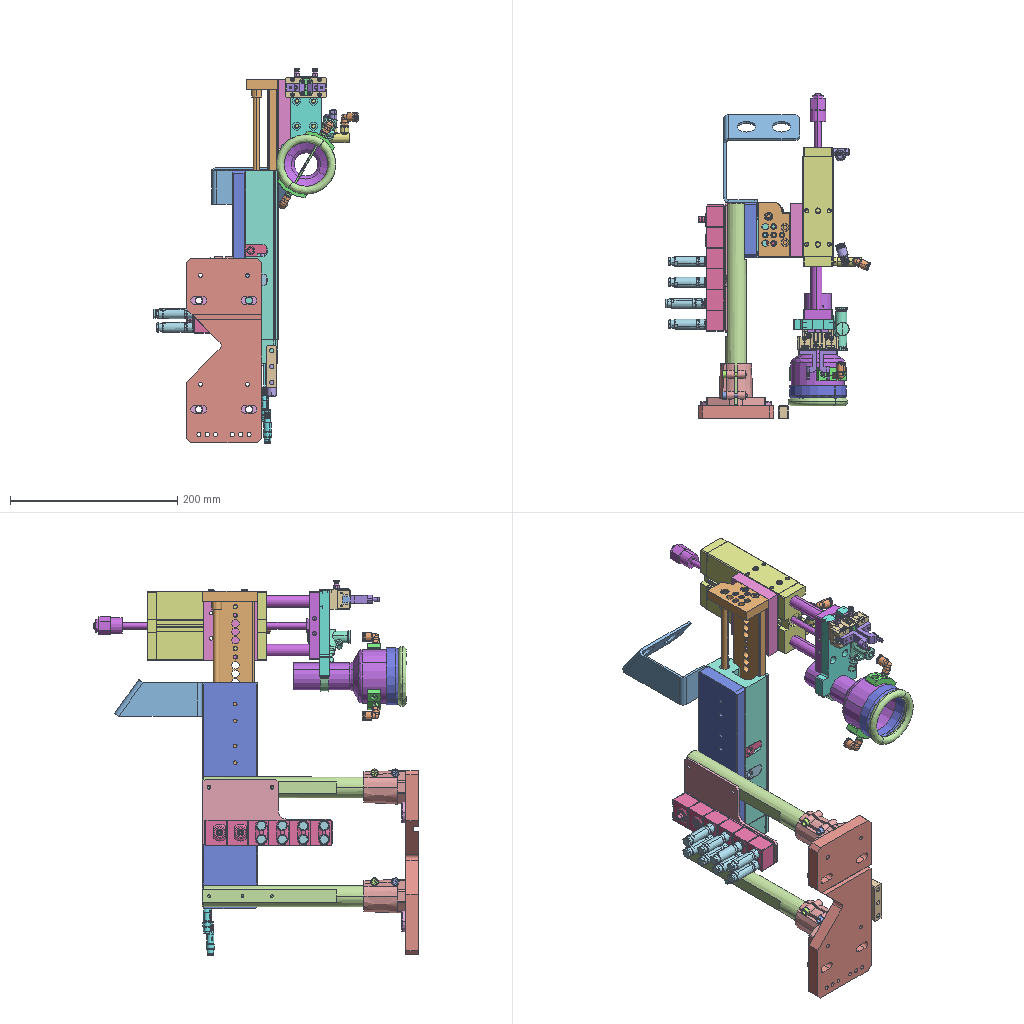Assembly | SolidWorks | 44 different items | 71 placed | box 245 x 388 x 448 mm
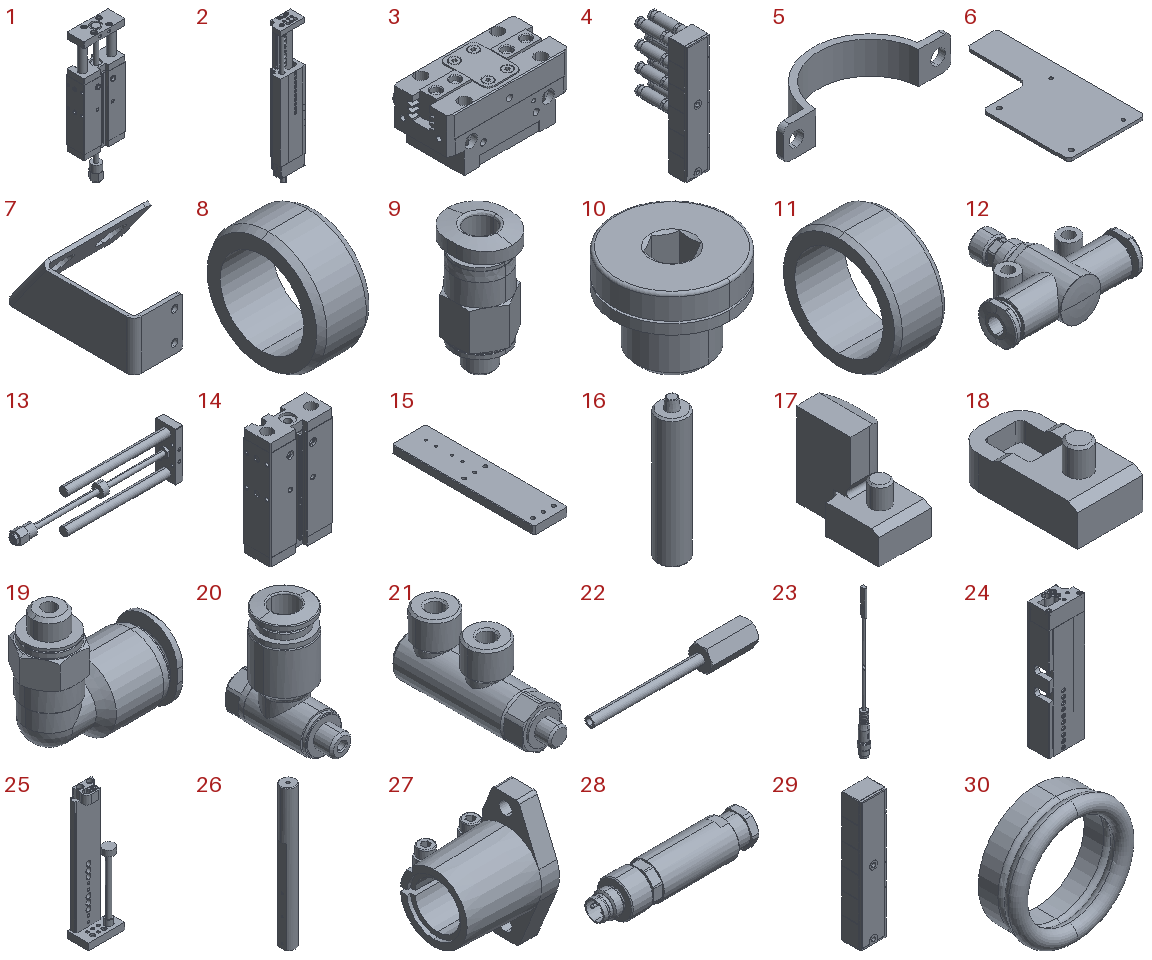Parts list (item | name | quantity | parent item | size | volume | features):
1 | (subassembly) | x1 | - | 84.4 x 37.9 x 271.9 mm | 422622 mm3 | -
2 | (subassembly) | x1 | - | 66 x 40 x 379 mm | 460415 mm3 | -
3 | (subassembly) | x1 | - | 50 x 34.8 x 24.7 mm | 23663 mm3 | -
4 | (subassembly) | x1 | - | 30 x 71.1 x 151 mm | 135395 mm3 | -
5 | - | x1 | - | 52 x 17 x 10 mm | 1282 mm3 | features ExtruThin 1, Fillet 1, HoleWzd 1
6 | - | x1 | - | 80 x 155 x 3 mm | 27690 mm3 | features HoleWzd 2, Chamfer 1, Extrusion 1, Fillet 1, ICE 1
7 | - | x1 | - | 91 x 104.854 x 43.527 mm | 25604 mm3 | features Fillet 2, ICE 2, EdgeFlange 1, FlatPattern 1, HoleWzd 1, SMBaseFlange 1, SheetMetal 1
8 | - | x4 | in 1 | 4 x 9 x 9 mm | 121.796 mm3 | features RefAxis 9, 3DProfileFeature 3, Revolution 1
9 | - | x2 | in 3 | 6 x 7 x 13.3 mm | 216.387 mm3 | features BaseBody 1
10 | - | x2 | in 2 | 8 x 8 x 6.3 mm | 181.471 mm3 | features RefAxis 6, 3DProfileFeature 2, ICE 1, Revolution 1
11 | - | x2 | in 1 | 3 x 7 x 7 mm | 48.144 mm3 | features RefAxis 9, 3DProfileFeature 3, Revolution 1
12 | - | x1 | - | 51.6 x 40.42 x 16.166 mm | 11359 mm3 | features BaseBody 1
13 | - | x1 | in 1 | 270 x 34 x 81 mm | 107228 mm3 | features RefAxis 9, RevCut 7, Revolution 6, ICE 4, 3DProfileFeature 3, HoleWzd 2, Extrusion 1
14 | - | x1 | in 1 | 83 x 36 x 142 mm | 314811 mm3 | features RefAxis 33, RevCut 25, 3DProfileFeature 11, ICE 4, Extrusion 1
15 | - | x1 | - | 66 x 270 x 15 mm | 261133 mm3 | features Chamfer 2, HoleWzd 2, ICE 2, Extrusion 1, MoveFace 1
16 | - | x2 | in 2 | 12 x 12 x 58.2 mm | 5676 mm3 | features RefAxis 21, 3DProfileFeature 7, Revolution 3, ICE 2, RevCut 2
17 | - | x1 | in 2 | 14 x 26.1 x 22.4 mm | 4263 mm3 | features ICE 6, RefAxis 3, 3DProfileFeature 1, Extrusion 1, RevCut 1, Revolution 1
18 | - | x1 | in 2 | 13.9 x 26.1 x 13.7 mm | 2228 mm3 | features ICE 4, RefAxis 3, 3DProfileFeature 1, Extrusion 1, RevCut 1, Revolution 1
19 | - | x3 | - | 20.919 x 10.5 x 20.4 mm | 1362 mm3 | features RefAxis 9, 3DProfileFeature 3, Revolution 3, ICE 2, RevCut 2
20 | - | x2 | - | 11.8 x 24.4 x 26.45 mm | 2431 mm3 | features BaseBody 1
21 | - | x1 | - | 11 x 39 x 19 mm | 4357 mm3 | features BaseBody 1
22 | - | x2 | - | 50 x 8.083 x 7 mm | 663.119 mm3 | features BaseBody 1
23 | - | x2 | - | 9.6 x 9.6 x 150.7 mm | 2540 mm3 | features Attribute 301, BaseBody 5, ICE 1
24 | - | x1 | in 2 | 66 x 39.6 x 230 mm | 297307 mm3 | features RefAxis 57, RevCut 21, 3DProfileFeature 19, ICE 16, Revolution 4, Extrusion 1
25 | - | x1 | in 2 | 65 x 38.5 x 229 mm | 144902 mm3 | features RevCut 22, RefAxis 18, ICE 12, 3DProfileFeature 6, Revolution 2, Extrusion 1
26 | - | x2 | - | 25 x 25 x 243 mm | 111932 mm3 | features HoleWzd 3, ICE 3, Chamfer 1, Extrusion 1
27 | - | x2 | - | 50 x 42 x 70 mm | 41488 mm3 | features BaseBody 3
28 | - | x8 | in 4 | 50.1 x 12 x 12 mm | 4699 mm3 | features BaseBody 1
29 | - | x1 | in 4 | 30 x 31.5 x 151 mm | 97801 mm3 | features BaseBody 1
30 | - | x1 | - | 71.5 x 24 x 71.5 mm | 15845 mm3 | features Sweep 2
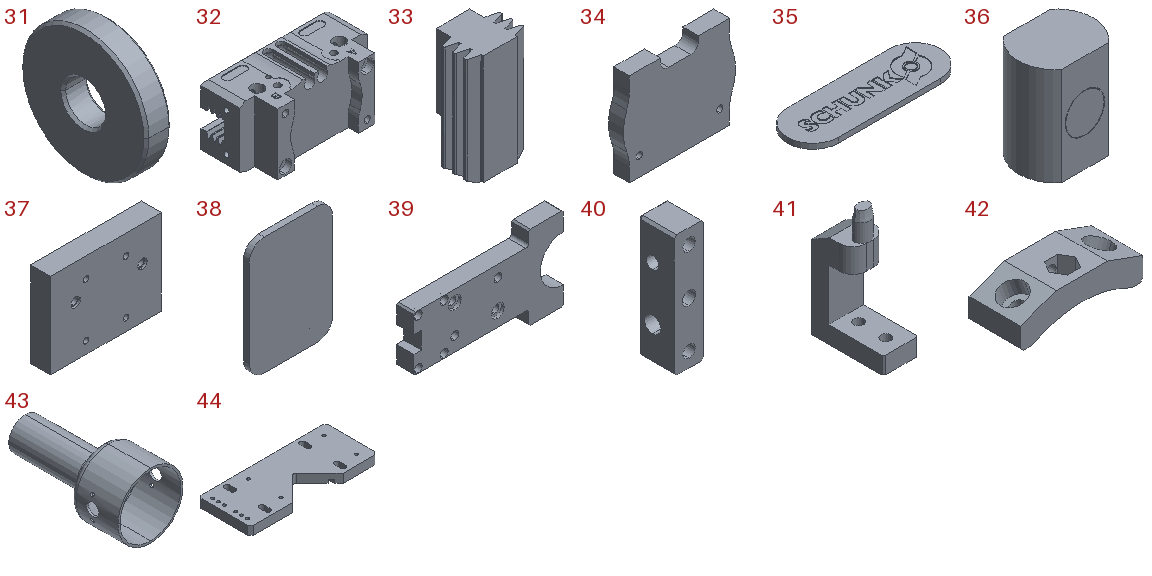31 | - | x4 | - | 5 x 25 x 25 mm | 2177 mm3 | features BaseBody 1
32 | - | x1 | in 3 | 50 x 24 x 25 mm | 17442 mm3 | features BaseBody 1
33 | - | x2 | in 3 | 11.68 x 9.5 x 22 mm | 1629 mm3 | features BaseBody 1
34 | - | x1 | in 3 | 27.8 x 3.9 x 23 mm | 2196 mm3 | features BaseBody 1
35 | - | x1 | in 3 | 9 x 3 x 0.3 mm | 7.24 mm3 | features BaseBody 1
36 | - | x1 | in 3 | 3.8 x 2.95 x 5 mm | 47.517 mm3 | features BaseBody 1
37 | - | x1 | - | 83 x 15 x 64 mm | 77222 mm3 | features HoleWzd 2, ICE 2, Extrusion 1
38 | - | x1 | in 3 | 14.4 x 1 x 20.4 mm | 279.954 mm3 | features BaseBody 1
39 | - | x1 | - | 104 x 12 x 58 mm | 44083 mm3 | features ICE 6, HoleWzd 3, Chamfer 1, Extrusion 1, Fillet 1
40 | - | x1 | - | 12 x 15 x 50 mm | 6990 mm3 | features HoleWzd 3, Chamfer 1, Extrusion 1, ICE 1
41 | - | x2 | - | 10 x 21 x 35 mm | 2531 mm3 | features ICE 4, Chamfer 3, Fillet 2, Extrusion 1, HoleWzd 1
42 | - | x2 | - | 38 x 16 x 11 mm | 3676 mm3 | features HoleWzd 2, Chamfer 1, Extrusion 1, ICE 1, MirrorPattern 1
43 | - | x1 | - | 64 x 123.238 x 64 mm | 34756 mm3 | features 3DProfileFeature 2, HoleWzd 2, Fillet 1, ICE 1, MirrorPattern 1, RefAxis 1, Revolution 1, Shell 1
44 | - | x1 | - | 220 x 90 x 15 mm | 252154 mm3 | features ICE 3, HoleWzd 2, Chamfer 1, Cut 1, Extrusion 1, Fillet 1
Mates (type | each side: item.copy, entity, surface, feature):
In the top assembly
Coincident | 27.1 face plane _SHFTL25_b-1-solid1 | 27.2 face plane _SHFTL25_b-1-solid1 | 2 times
Concentric | 26.1 face cylinder Boss-Extrude1 | 27.1 face cylinder _SHFTL25_b-1-solid1
Concentric | 26.2 face cylinder Boss-Extrude1 | 27.2 face cylinder _SHFTL25_b-1-solid1
Coincident | 15.1 face plane Boss-Extrude1 | 24.1 face plane Boss-Extrude2 | 3 times
Coincident | 26.2 face plane Cut-Extrude1 | 15.1 face plane Boss-Extrude1
Coincident | 26.1 face plane Cut-Extrude1 | 15.1 face plane Boss-Extrude1
Concentric | 26.1 face cylinder M6 Tapped Hole2 | 15.1 face cylinder CBORE for M6 Hex Socket Head Cap Screw1 | 2 times
Concentric | 26.2 face cylinder M6 Tapped Hole2 | 15.1 face cylinder CBORE for M6 Hex Socket Head Cap Screw1
Concentric | 23.1 face cylinder Input 1 | 24.1 face cylinder Boss-Extrude2
Concentric | 23.2 face cylinder Input 1 | 24.1 face cylinder Boss-Extrude2
Parallel | 23.1 face plane Input 1 | 24.1 face plane Boss-Extrude2
Parallel | 23.2 face plane Input 1 | 24.1 face plane Boss-Extrude2
Coincident | 37.1 face plane Boss-Extrude1 | 25.1 face plane Boss-Extrude2
Coincident | 37.1 face plane Boss-Extrude1 | 25.1 face plane Boss-Extrude1 | 2 times
Coincident | 37.1 face plane Boss-Extrude1 | 14.1 face plane Boss-Extrude1 | 3 times
Concentric | 20.1 face cylinder Input 1 | 14.1 face cylinder Cut-Revolve16
Coincident | 20.1 face plane Input 1 | 14.1 face plane Boss-Extrude2
Coincident | 39.1 face plane Boss-Extrude1 | 13.1 face plane Boss-Extrude1
Width | 13.1 face plane Boss-Extrude1 | 13.1 face plane Boss-Extrude1 | 39.1 face plane Boss-Extrude1 | 39.1 face plane Boss-Extrude1
Coincident | 15.1 face plane Boss-Extrude1 | assembly plane | 3 times
Coincident | 23.2 face plane Input 1 | 23.1 face plane Input 1
Coincident | 23.2 face plane Input 1 | 24.1 face plane Boss-Extrude2
Coincident | 26.2 face plane Boss-Extrude1 | 27.2 face plane _SHFTL25_b-1-solid1
Coincident | 27.2 face plane _SHFTL25_b-1-solid1 | 44.1 face plane Boss-Extrude1
Concentric | 27.2 face cylinder _SHFTL25_b-1-solid1 | 44.1 face cylinder M6 Tapped Hole1
Concentric | 27.1 face cylinder _SHFTL25_b-1-solid1 | 44.1 face cylinder M6 Tapped Hole1
Coincident | 44.1 face plane Boss-Extrude1 | 40.1 face plane Boss-Extrude1
DistanceDim | 44.1 face plane Boss-Extrude1 | 40.1 face plane Boss-Extrude1
Concentric | 44.1 face cylinder M6 Tapped Hole2 | 40.1 face cylinder M6 Clearance Hole2
Coincident | 44.1 select_type:24 | 31.1 face cylinder Input 1
Coincident | 44.1 face plane Boss-Extrude1 | 31.1 face plane Input 1
Coincident | 44.1 select_type:24 | 31.2 face cylinder Input 1
Coincident | 44.1 face plane Boss-Extrude1 | 31.2 face plane Input 1
Coincident | 44.1 select_type:24 | 31.3 face cylinder Input 1
Coincident | 44.1 face plane Boss-Extrude1 | 31.3 face plane Input 1
Coincident | 44.1 select_type:24 | 31.4 face cylinder Input 1
Coincident | 44.1 face plane Boss-Extrude1 | 31.4 face plane Input 1
Coincident | 39.1 face plane Boss-Extrude1 | 32.1 face plane Input 1 | 2 times
Width | 32.1 face plane Input 1 | 32.1 face plane Input 1 | 39.1 face plane Boss-Extrude1 | 39.1 face plane Boss-Extrude1
Concentric | 33.1 face cylinder Input 1 | 41.1 face cylinder M2.5 Clearance Hole1 | 2 times
Concentric | 33.2 face cylinder Input 1 | 41.2 face cylinder M2.5 Clearance Hole1 | 2 times
Coincident | 33.1 face plane Input 1 | 41.1 face plane Boss-Extrude1
Coincident | 33.2 face plane Input 1 | 41.2 face plane Boss-Extrude1
Concentric | 43.1 face cylinder Revolve1 | 5.1 face cylinder Extrude-Thin1
Concentric | 43.1 face cylinder Revolve1 | 30.1 face cylinder Sweep1
Tangent | 43.1 face plane Revolve1 | 30.1 face torus Sweep1
DistanceDim | 43.1 face plane Revolve1 | 5.1 face plane Extrude-Thin1
Concentric | 19.1 face cylinder Cut-Revolve2 | 12.1 face cylinder Input 1
DistanceDim | 12.1 face plane Input 1 | 19.1 face plane Revolve1
Concentric | 39.1 face cylinder Cut-Extrude2 | 43.1 face cylinder Revolve1
Parallel | 39.1 face plane Boss-Extrude1 | 5.1 face plane Extrude-Thin1
Concentric | 39.1 face cylinder M4 Tapped Hole1 | 5.1 face cylinder M4 Clearance Hole1
Concentric | 14.1 face cylinder Cut-Revolve15 | 21.1 face cylinder Input 1
Coincident | 14.1 face plane Boss-Extrude3 | 21.1 face plane Input 1
Concentric | 20.2 face cylinder Input 1 | 21.1 face cylinder Input 1
Coincident | 20.2 face plane Input 1 | 21.1 face plane Input 1
Concentric | 21.1 face cylinder Input 1 | 19.2 face cylinder Revolve3
Coincident | 21.1 face plane Input 1 | 19.2 face plane Revolve2
Concentric | 43.1 face cylinder M4 Tapped Hole1 | 42.1 face cylinder Mirror3
Concentric | 43.1 face cylinder M4 Tapped Hole1 | 42.1 face cylinder Hole size per socket head cap screw type 2
Concentric | 43.1 face cylinder Cut-Extrude1 | 22.1 face cylinder Input 1
Parallel | 42.1 face plane Cut-Extrude2 | 22.1 face plane Input 1
DistanceDim | 22.1 face plane Input 1 | 42.1 face plane Boss-Extrude1
Concentric | 19.3 face cylinder Revolve3 | 22.1 face cylinder Input 1
Coincident | 19.3 face plane Revolve2 | 22.1 face plane Input 1
Parallel | 42.2 face plane Cut-Extrude2 | 22.2 face plane Input 1
DistanceDim | 22.2 face plane Input 1 | 42.2 face plane Boss-Extrude1
Concentric | 43.1 face cylinder M4 Tapped Hole1 | 42.2 face cylinder Mirror3
Concentric | 43.1 face cylinder M4 Tapped Hole1 | 42.2 face cylinder Hole size per socket head cap screw type 2
Concentric | 43.1 face cylinder Cut-Extrude1 | 22.2 face cylinder Input 1
Concentric | 19.1 face cylinder Revolve3 | 22.2 face cylinder Input 1
Coincident | 19.1 face plane Revolve2 | 22.2 face plane Input 1
DistanceDim | 13.1 face plane Boss-Extrude1 | 39.1 face plane Boss-Extrude1
DistanceDim | 42.2 edge | 39.1 face plane Boss-Extrude2
Concentric | 26.2 face cylinder M4 Tapped Hole1 | 6.1 face cylinder M4 Clearance Hole1 | 2 times
Coincident | 26.2 face plane Cut-Extrude2 | 6.1 face plane Boss-Extrude1
Concentric | 29.1 face cylinder Input 1 | 6.1 face cylinder M4 Tapped Hole1 | 2 times
Coincident | 29.1 face plane Input 1 | 6.1 face plane Boss-Extrude1
Coincident | 15.1 face plane Boss-Extrude1 | 7.1 face plane Base-Flange1 | 2 times
Coincident | 24.1 face plane Boss-Extrude2 | 7.1 face plane Base-Flange1
In subassembly 1
Coincident | 14.2 axis | 13.2 axis
PlanarAngleDim | 13.2 plane | 14.2 plane
DistanceDim | 8.1 plane | 13.2 plane
Coincident | 13.2 axis | 8.1 axis
PlanarAngleDim | 8.1 plane | 13.2 plane
DistanceDim | 8.2 plane | 13.2 plane
Coincident | 13.2 axis | 8.2 axis
PlanarAngleDim | 8.2 plane | 13.2 plane
DistanceDim | 8.3 plane | 14.2 plane
Coincident | 14.2 axis | 8.3 axis
PlanarAngleDim | 8.3 plane | 14.2 plane
DistanceDim | 8.4 plane | 14.2 plane
Coincident | 14.2 axis | 8.4 axis
PlanarAngleDim | 8.4 plane | 14.2 plane
DistanceDim | 11.1 plane | 14.2 plane
Coincident | 14.2 axis | 11.1 axis
PlanarAngleDim | 11.1 plane | 14.2 plane
DistanceDim | 11.2 plane | 14.2 plane
Coincident | 14.2 axis | 11.2 axis
PlanarAngleDim | 11.2 plane | 14.2 plane
LimitDistanceDim | 14.2 face plane Cut-Revolve22 | 13.2 face plane Revolve3
In subassembly 2
Coincident | 24.2 axis | 25.2 axis
PlanarAngleDim | 25.2 plane | 24.2 plane
DistanceDim | 16.1 plane | 25.2 plane
Coincident | 25.2 axis | 16.1 axis
PlanarAngleDim | 16.1 plane | 25.2 plane
DistanceDim | 16.2 plane | 24.2 plane
Coincident | 24.2 axis | 16.2 axis
PlanarAngleDim | 16.2 plane | 24.2 plane
DistanceDim | 10.1 plane | 24.2 plane
Coincident | 24.2 axis | 10.1 axis
PlanarAngleDim | 10.1 plane | 24.2 plane
DistanceDim | 10.2 plane | 24.2 plane
Coincident | 24.2 axis | 10.2 axis
PlanarAngleDim | 10.2 plane | 24.2 plane
DistanceDim | 17.1 plane | 24.2 plane
Coincident | 24.2 axis | 17.1 axis
PlanarAngleDim | 17.1 plane | 24.2 plane
DistanceDim | 18.1 plane | 24.2 plane
Coincident | 24.2 axis | 18.1 axis
PlanarAngleDim | 18.1 plane | 24.2 plane
LimitDistanceDim | 25.2 face plane Revolve1 | 24.2 face plane Cut-Revolve7
In subassembly 3
Width | 32.2 face plane Input 1 | 32.2 face plane Input 1 | 33.3 face plane Input 1 | 33.3 face plane Input 1
DistanceDim | 33.3 face plane Input 1 | 32.2 face plane Input 1
Coincident | 33.3 face plane Input 1 | 33.4 face plane Input 1 | 2 times
Width | 33.3 face plane Input 1 | 33.4 face plane Input 1 | 32.2 face plane Input 1 | 32.2 face plane Input 1
LimitDistanceDim | 33.3 face plane Input 1 | 33.4 face plane Input 1
Concentric | 32.2 face cylinder Input 1 | 9.1 face cylinder Input 1
Coincident | 32.2 face plane Input 1 | 9.1 face plane Input 1
Concentric | 32.2 face cylinder Input 1 | 9.2 face cylinder Input 1
Coincident | 32.2 face plane Input 1 | 9.2 face plane Input 1
In subassembly 4
Concentric | 28.1 face cylinder Input 1 | 29.2 face cylinder Input 1
Coincident | 29.2 face plane Input 1 | 28.1 face plane Input 1
Concentric | 29.2 face cylinder Input 1 | 28.2 face cylinder Input 1
Concentric | 29.2 face cylinder Input 1 | 28.3 face cylinder Input 1
Concentric | 29.2 face cylinder Input 1 | 28.4 face cylinder Input 1
Concentric | 29.2 face cylinder Input 1 | 28.5 face cylinder Input 1
Concentric | 29.2 face cylinder Input 1 | 28.6 face cylinder Input 1
Concentric | 29.2 face cylinder Input 1 | 28.7 face cylinder Input 1
Concentric | 29.2 face cylinder Input 1 | 28.8 face cylinder Input 1
Coincident | 29.2 face plane Input 1 | 28.5 face plane Input 1
Coincident | 28.1 face plane Input 1 | 28.2 face plane Input 1
Coincident | 28.1 face plane Input 1 | 28.4 face plane Input 1
Coincident | 28.1 face plane Input 1 | 28.3 face plane Input 1
Coincident | 28.1 face plane Input 1 | 28.8 face plane Input 1
Coincident | 28.1 face plane Input 1 | 28.7 face plane Input 1
Coincident | 28.1 face plane Input 1 | 28.6 face plane Input 1